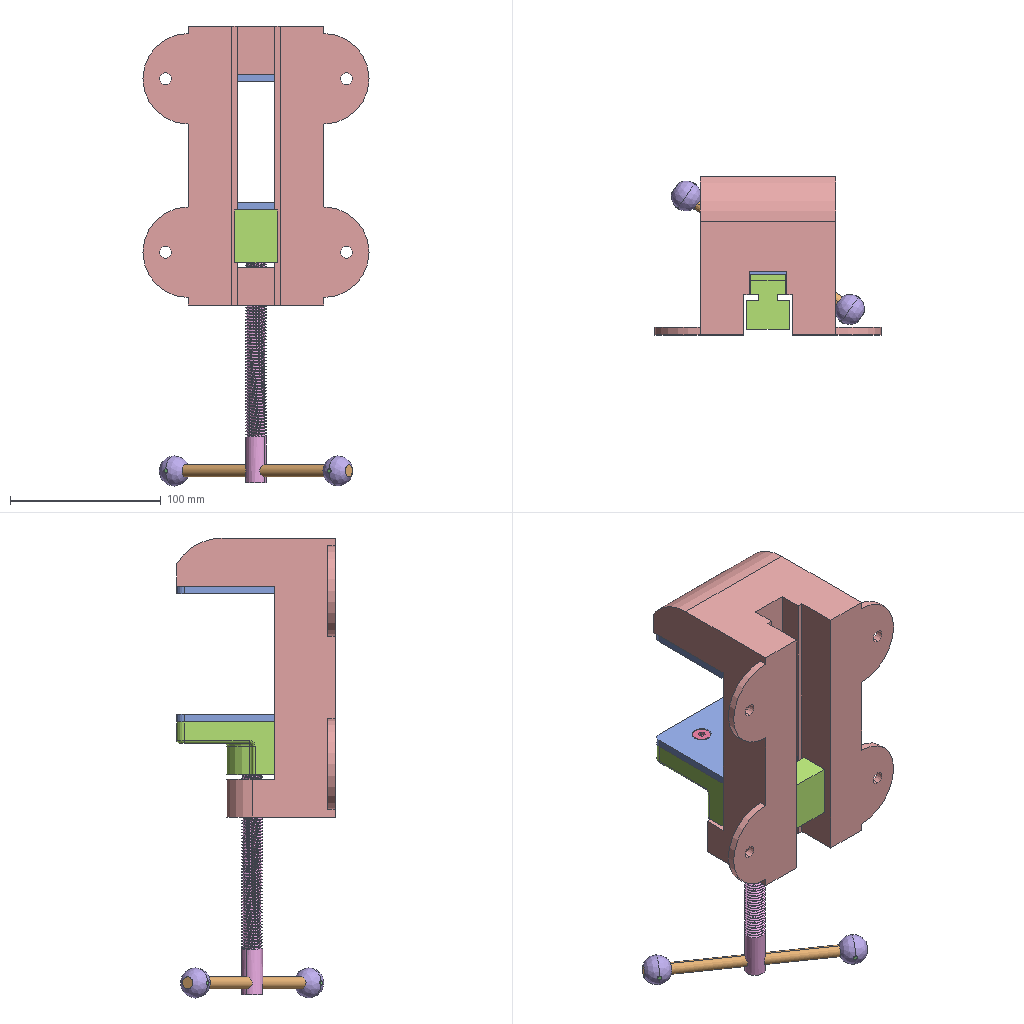Assembly | SolidWorks | 10 different items | 12 placed | box 150 x 105 x 305 mm
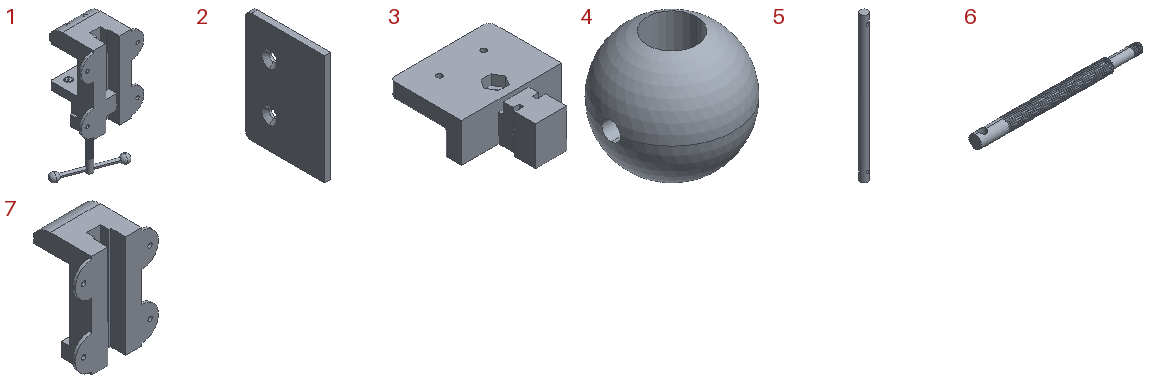Parts list (item | name | quantity | size | volume | features):
1 | (subassembly) | x1 | 150 x 105 x 303.032 mm | 931292 mm3 | features MirrorCompFeat 2, CompositeCurve 1, ReferencePattern 1
2 | - | x2 | 5 x 65 x 90 mm | 28593 mm3 | features Extrusion 1, HoleWzd 1
3 | - | x1 | 90 x 101 x 35 mm | 144752 mm3 | features ICE 3, Cut 1, Extrusion 1, Fillet 1, HoleWzd 1
4 | - | x2 | 19.774 x 20 x 18.33 mm | 3140 mm3 | features ICE 2, Revolution 1
5 | - | x1 | 8 x 8 x 150 mm | 7429 mm3 | features Extrusion 1, ICE 1
6 | - | x1 | 180 x 13.8 x 13.8 mm | 20623 mm3 | features ICE 3, Chamfer 2, Helix 2, SweepCut 2, Revolution 1
7 | - | x1 | 150 x 105 x 185 mm | 685281 mm3 | features ICE 3, Extrusion 1, Helix 1, HoleWzd 1, SweepCut 1
8 | hex lobular socket ctsk screws gb | x1 | - | - | -
9 | hex nuts, style 1-grades ab gb | x1 | - | - | -
10 | parallel pins unhardening steel gb | x1 | - | - | -
Mates (type | each side: item.copy, entity, surface, feature):
Coincident | 7.1 plane | assembly plane | 3 times
Coincident | 7.1 face plane Boss-Extrude1 | 2.1 face plane Boss-Extrude1 | 2 times
Concentric | 7.1 face cylinder M6 Tapped Hole1 | 2.1 face cylinder Hole size by hex socket countersunk screw type1
Parallel | 7.1 face plane Boss-Extrude1 | 2.1 face plane Boss-Extrude1
Width | 3.1 face plane Extrude1 | 3.1 face plane Extrude1 | 7.1 face plane Cut-Extrude1 | 7.1 face plane Cut-Extrude1
Coincident | 7.1 face plane Boss-Extrude1 | 3.1 face plane Extrude1
Coincident | 3.1 face plane Extrude2 | 2.2 face plane Boss-Extrude1
Concentric | 3.1 face cylinder M6 Tapped Hole2 | 2.2 face cylinder Hole size by hex socket countersunk screw type1
Coincident | 3.1 face plane Extrude1 | 2.2 face plane Boss-Extrude1
Concentric | 3.1 face cylinder Cut-Extrude1 | 6.1 face cylinder Revolve1
Coincident | 3.1 face plane Extrude1 | 6.1 face plane Revolve1
LimitDistanceDim | 2.1 face plane Boss-Extrude1 | 2.2 face plane Boss-Extrude1
Coincident | 6.1 axis | 5.1 axis
Parallel | 6.1 face plane Revolve1 | 5.1 plane
Coincident | 6.1 axis | 5.1 plane
Screw | 7.1 face cylinder Cut-Extrude2 | 6.1 face cylinder Revolve1
Concentric | 5.1 face cylinder Boss-Extrude1 | 4.1 face cylinder Cut-Extrude1
Coincident | 5.1 axis | 4.1 axis
Coincident | 5.1 axis | 4.2 axis | 2 times